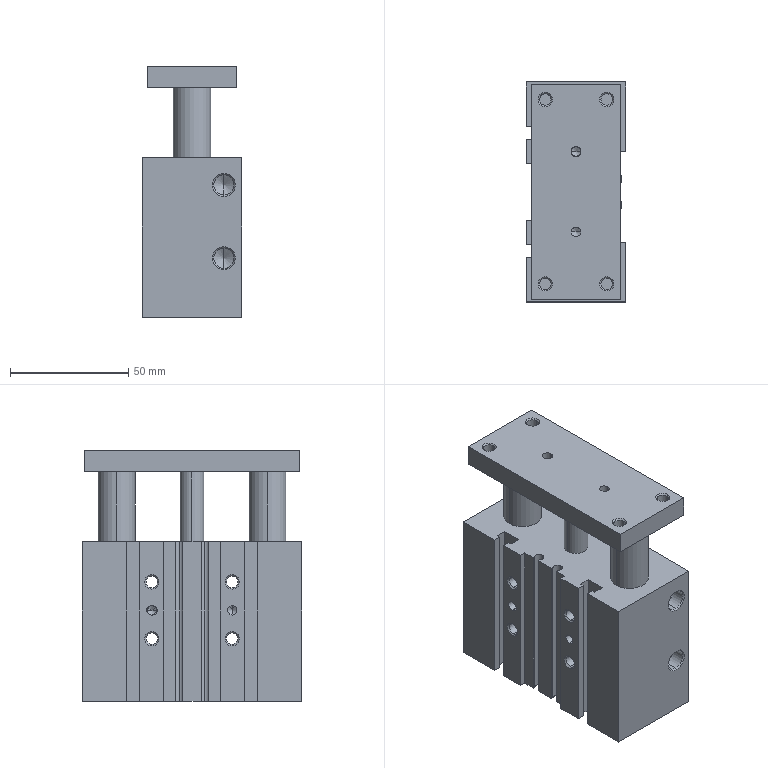Part | SolidWorks | 6 solids | 271 faces | box 42 x 93 x 106.033 mm | volume 253886 mm3 | cylinder 105 | plane 98 | cone 68 | commonest cylinder face diameters 4.917 x24 4 x21 5.4 x8 8.566 x8 9.5 x8 16 x8